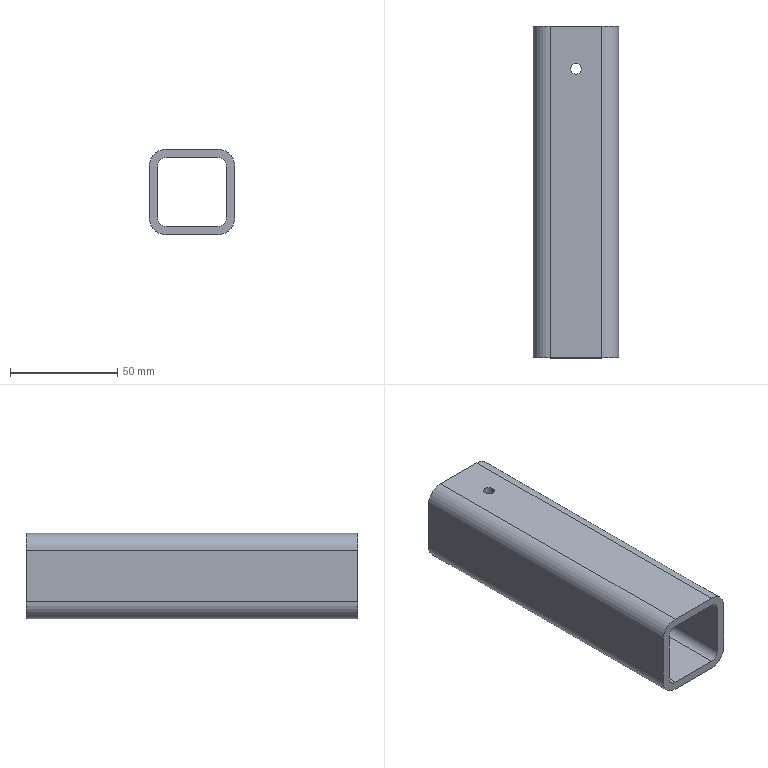Part | SolidWorks | features HoleWzd 1, WeldMemberFeat 1, WeldmentFeature 1 | 1 solid | 22 faces | box 40 x 155 x 40 mm | volume 82736 mm3 | cylinder 12 | plane 10 | commonest cylinder face diameters 5 x4 8 x4 16 x4
STEP:
#1=CARTESIAN_POINT('',(2.5,135.,16.));
#2=VERTEX_POINT('',#1);
#3=CARTESIAN_POINT('',(-2.5,135.,16.));
#4=VERTEX_POINT('',#3);
#5=CARTESIAN_POINT('',(0.,135.,16.));
#6=DIRECTION('',(0.,0.,-1.));
#7=DIRECTION('',(-1.,0.,0.));
#8=AXIS2_PLACEMENT_3D('',#5,#6,#7);
#9=CIRCLE('',#8,2.5);
#10=EDGE_CURVE('',#2,#4,#9,.T.);
#11=ORIENTED_EDGE('',*,*,#10,.T.);
#12=CARTESIAN_POINT('',(-2.5,135.,20.));
#13=VERTEX_POINT('',#12);
#14=CARTESIAN_POINT('',(-2.5,135.,20.));
#15=DIRECTION('',(0.,0.,1.));
#16=VECTOR('',#15,1000.);
#17=LINE('',#14,#16);
#18=EDGE_CURVE('',#4,#13,#17,.T.);
#19=ORIENTED_EDGE('',*,*,#18,.T.);
#20=CARTESIAN_POINT('',(2.5,135.,20.));
#21=VERTEX_POINT('',#20);
#22=CARTESIAN_POINT('',(0.,135.,20.));
#23=DIRECTION('',(0.,0.,1.));
#24=DIRECTION('',(1.,0.,0.));
#25=AXIS2_PLACEMENT_3D('',#22,#23,#24);
#26=CIRCLE('',#25,2.5);
#27=EDGE_CURVE('',#13,#21,#26,.T.);
#28=ORIENTED_EDGE('',*,*,#27,.T.);
#29=CARTESIAN_POINT('',(2.5,135.,20.));
#30=DIRECTION('',(0.,0.,1.));
#31=VECTOR('',#30,1000.);
#32=LINE('',#29,#31);
#33=EDGE_CURVE('',#2,#21,#32,.T.);
#34=ORIENTED_EDGE('',*,*,#33,.F.);
#35=EDGE_LOOP('',(#11,#19,#28,#34));
#36=FACE_OUTER_BOUND('',#35,.T.);
#37=CARTESIAN_POINT('',(0.,135.,20.));
#38=DIRECTION('',(0.,0.,1.));
#39=DIRECTION('',(1.,0.,0.));
#40=AXIS2_PLACEMENT_3D('',#37,#38,#39);
#41=CYLINDRICAL_SURFACE('',#40,2.5);
#42=ADVANCED_FACE('',(#36),#41,.F.);
#43=CARTESIAN_POINT('',(-2.5,135.,-20.));
#44=VERTEX_POINT('',#43);
#45=CARTESIAN_POINT('',(2.5,135.,-20.));
#46=VERTEX_POINT('',#45);
#47=CARTESIAN_POINT('',(0.,135.,-20.));
#48=DIRECTION('',(0.,0.,1.));
#49=DIRECTION('',(1.,0.,0.));
#50=AXIS2_PLACEMENT_3D('',#47,#48,#49);
#51=CIRCLE('',#50,2.5);
#52=EDGE_CURVE('',#44,#46,#51,.T.);
#53=ORIENTED_EDGE('',*,*,#52,.F.);
#54=CARTESIAN_POINT('',(-2.5,135.,-16.));
#55=VERTEX_POINT('',#54);
#56=CARTESIAN_POINT('',(-2.5,135.,20.));
#57=DIRECTION('',(0.,0.,1.));
#58=VECTOR('',#57,1000.);
#59=LINE('',#56,#58);
#60=EDGE_CURVE('',#44,#55,#59,.T.);
#61=ORIENTED_EDGE('',*,*,#60,.T.);
#62=CARTESIAN_POINT('',(2.5,135.,-16.));
#63=VERTEX_POINT('',#62);
#64=CARTESIAN_POINT('',(0.,135.,-16.));
#65=DIRECTION('',(0.,0.,1.));
#66=DIRECTION('',(1.,0.,0.));
#67=AXIS2_PLACEMENT_3D('',#64,#65,#66);
#68=CIRCLE('',#67,2.5);
#69=EDGE_CURVE('',#55,#63,#68,.T.);
#70=ORIENTED_EDGE('',*,*,#69,.T.);
#71=CARTESIAN_POINT('',(2.5,135.,20.));
#72=DIRECTION('',(0.,0.,1.));
#73=VECTOR('',#72,1000.);
#74=LINE('',#71,#73);
#75=EDGE_CURVE('',#46,#63,#74,.T.);
#76=ORIENTED_EDGE('',*,*,#75,.F.);
#77=EDGE_LOOP('',(#53,#61,#70,#76));
#78=FACE_OUTER_BOUND('',#77,.T.);
#79=CARTESIAN_POINT('',(0.,135.,20.));
#80=DIRECTION('',(0.,0.,1.));
#81=DIRECTION('',(1.,0.,0.));
#82=AXIS2_PLACEMENT_3D('',#79,#80,#81);
#83=CYLINDRICAL_SURFACE('',#82,2.5);
#84=ADVANCED_FACE('',(#78),#83,.F.);
#85=CARTESIAN_POINT('',(20.,155.,12.));
#86=VERTEX_POINT('',#85);
#87=CARTESIAN_POINT('',(12.,155.,20.));
#88=VERTEX_POINT('',#87);
#89=CARTESIAN_POINT('',(12.,155.,12.));
#90=DIRECTION('',(0.,-1.,0.));
#91=DIRECTION('',(1.,0.,0.));
#92=AXIS2_PLACEMENT_3D('',#89,#90,#91);
#93=CIRCLE('',#92,8.);
#94=EDGE_CURVE('',#86,#88,#93,.T.);
#95=ORIENTED_EDGE('',*,*,#94,.T.);
#96=CARTESIAN_POINT('',(12.,0.,20.));
#97=VERTEX_POINT('',#96);
#98=CARTESIAN_POINT('',(12.,0.,20.));
#99=DIRECTION('',(0.,1.,0.));
#100=VECTOR('',#99,1000.);
#101=LINE('',#98,#100);
#102=EDGE_CURVE('',#97,#88,#101,.T.);
#103=ORIENTED_EDGE('',*,*,#102,.F.);
#104=CARTESIAN_POINT('',(20.,0.,12.));
#105=VERTEX_POINT('',#104);
#106=CARTESIAN_POINT('',(12.,0.,12.));
#107=DIRECTION('',(0.,-1.,0.));
#108=DIRECTION('',(1.,0.,0.));
#109=AXIS2_PLACEMENT_3D('',#106,#107,#108);
#110=CIRCLE('',#109,8.);
#111=EDGE_CURVE('',#105,#97,#110,.T.);
#112=ORIENTED_EDGE('',*,*,#111,.F.);
#113=CARTESIAN_POINT('',(20.,0.,12.));
#114=DIRECTION('',(0.,1.,0.));
#115=VECTOR('',#114,1000.);
#116=LINE('',#113,#115);
#117=EDGE_CURVE('',#105,#86,#116,.T.);
#118=ORIENTED_EDGE('',*,*,#117,.T.);
#119=EDGE_LOOP('',(#95,#103,#112,#118));
#120=FACE_OUTER_BOUND('',#119,.T.);
#121=CARTESIAN_POINT('',(12.,0.,12.));
#122=DIRECTION('',(0.,1.,0.));
#123=DIRECTION('',(-1.,0.,0.));
#124=AXIS2_PLACEMENT_3D('',#121,#122,#123);
#125=CYLINDRICAL_SURFACE('',#124,8.);
#126=ADVANCED_FACE('',(#120),#125,.T.);
#127=CARTESIAN_POINT('',(0.,135.,20.));
#128=DIRECTION('',(0.,0.,1.));
#129=DIRECTION('',(1.,0.,0.));
#130=AXIS2_PLACEMENT_3D('',#127,#128,#129);
#131=CIRCLE('',#130,2.5);
#132=EDGE_CURVE('',#21,#13,#131,.T.);
#133=ORIENTED_EDGE('',*,*,#132,.F.);
#134=ORIENTED_EDGE('',*,*,#27,.F.);
#135=EDGE_LOOP('',(#133,#134));
#136=FACE_BOUND('',#135,.T.);
#137=CARTESIAN_POINT('',(-12.,155.,20.));
#138=VERTEX_POINT('',#137);
#139=CARTESIAN_POINT('',(12.,155.,20.));
#140=DIRECTION('',(-1.,0.,0.));
#141=VECTOR('',#140,1000.);
#142=LINE('',#139,#141);
#143=EDGE_CURVE('',#88,#138,#142,.T.);
#144=ORIENTED_EDGE('',*,*,#143,.T.);
#145=CARTESIAN_POINT('',(-12.,0.,20.));
#146=VERTEX_POINT('',#145);
#147=CARTESIAN_POINT('',(-12.,0.,20.));
#148=DIRECTION('',(0.,1.,0.));
#149=VECTOR('',#148,1000.);
#150=LINE('',#147,#149);
#151=EDGE_CURVE('',#146,#138,#150,.T.);
#152=ORIENTED_EDGE('',*,*,#151,.F.);
#153=CARTESIAN_POINT('',(12.,0.,20.));
#154=DIRECTION('',(-1.,0.,0.));
#155=VECTOR('',#154,1000.);
#156=LINE('',#153,#155);
#157=EDGE_CURVE('',#97,#146,#156,.T.);
#158=ORIENTED_EDGE('',*,*,#157,.F.);
#159=ORIENTED_EDGE('',*,*,#102,.T.);
#160=EDGE_LOOP('',(#144,#152,#158,#159));
#161=FACE_OUTER_BOUND('',#160,.T.);
#162=CARTESIAN_POINT('',(12.,0.,20.));
#163=DIRECTION('',(0.,0.,-1.));
#164=DIRECTION('',(-1.,0.,0.));
#165=AXIS2_PLACEMENT_3D('',#162,#163,#164);
#166=PLANE('',#165);
#167=ADVANCED_FACE('',(#136,#161),#166,.F.);
#168=CARTESIAN_POINT('',(-20.,155.,12.));
#169=VERTEX_POINT('',#168);
#170=CARTESIAN_POINT('',(-12.,155.,12.));
#171=DIRECTION('',(0.,-1.,0.));
#172=DIRECTION('',(1.,0.,0.));
#173=AXIS2_PLACEMENT_3D('',#170,#171,#172);
#174=CIRCLE('',#173,8.);
#175=EDGE_CURVE('',#138,#169,#174,.T.);
#176=ORIENTED_EDGE('',*,*,#175,.T.);
#177=CARTESIAN_POINT('',(-20.,0.,12.));
#178=VERTEX_POINT('',#177);
#179=CARTESIAN_POINT('',(-20.,0.,12.));
#180=DIRECTION('',(0.,1.,0.));
#181=VECTOR('',#180,1000.);
#182=LINE('',#179,#181);
#183=EDGE_CURVE('',#178,#169,#182,.T.);
#184=ORIENTED_EDGE('',*,*,#183,.F.);
#185=CARTESIAN_POINT('',(-12.,0.,12.));
#186=DIRECTION('',(0.,-1.,0.));
#187=DIRECTION('',(1.,0.,0.));
#188=AXIS2_PLACEMENT_3D('',#185,#186,#187);
#189=CIRCLE('',#188,8.);
#190=EDGE_CURVE('',#146,#178,#189,.T.);
#191=ORIENTED_EDGE('',*,*,#190,.F.);
#192=ORIENTED_EDGE('',*,*,#151,.T.);
#193=EDGE_LOOP('',(#176,#184,#191,#192));
#194=FACE_OUTER_BOUND('',#193,.T.);
#195=CARTESIAN_POINT('',(-12.,0.,12.));
#196=DIRECTION('',(0.,1.,0.));
#197=DIRECTION('',(-1.,0.,0.));
#198=AXIS2_PLACEMENT_3D('',#195,#196,#197);
#199=CYLINDRICAL_SURFACE('',#198,8.);
#200=ADVANCED_FACE('',(#194),#199,.T.);
#201=CARTESIAN_POINT('',(-20.,155.,-12.));
#202=VERTEX_POINT('',#201);
#203=CARTESIAN_POINT('',(-20.,155.,-12.));
#204=DIRECTION('',(0.,0.,-1.));
#205=VECTOR('',#204,1000.);
#206=LINE('',#203,#205);
#207=EDGE_CURVE('',#169,#202,#206,.T.);
#208=ORIENTED_EDGE('',*,*,#207,.T.);
#209=CARTESIAN_POINT('',(-20.,0.,-12.));
#210=VERTEX_POINT('',#209);
#211=CARTESIAN_POINT('',(-20.,0.,-12.));
#212=DIRECTION('',(0.,1.,0.));
#213=VECTOR('',#212,1000.);
#214=LINE('',#211,#213);
#215=EDGE_CURVE('',#210,#202,#214,.T.);
#216=ORIENTED_EDGE('',*,*,#215,.F.);
#217=CARTESIAN_POINT('',(-20.,0.,-12.));
#218=DIRECTION('',(0.,0.,-1.));
#219=VECTOR('',#218,1000.);
#220=LINE('',#217,#219);
#221=EDGE_CURVE('',#178,#210,#220,.T.);
#222=ORIENTED_EDGE('',*,*,#221,.F.);
#223=ORIENTED_EDGE('',*,*,#183,.T.);
#224=EDGE_LOOP('',(#208,#216,#222,#223));
#225=FACE_OUTER_BOUND('',#224,.T.);
#226=CARTESIAN_POINT('',(-20.,0.,-12.));
#227=DIRECTION('',(1.,0.,0.));
#228=DIRECTION('',(0.,1.,0.));
#229=AXIS2_PLACEMENT_3D('',#226,#227,#228);
#230=PLANE('',#229);
#231=ADVANCED_FACE('',(#225),#230,.F.);
#232=CARTESIAN_POINT('',(-12.,155.,-20.));
#233=VERTEX_POINT('',#232);
#234=CARTESIAN_POINT('',(-12.,155.,-12.));
#235=DIRECTION('',(0.,-1.,0.));
#236=DIRECTION('',(1.,0.,0.));
#237=AXIS2_PLACEMENT_3D('',#234,#235,#236);
#238=CIRCLE('',#237,8.);
#239=EDGE_CURVE('',#202,#233,#238,.T.);
#240=ORIENTED_EDGE('',*,*,#239,.T.);
#241=CARTESIAN_POINT('',(-12.,0.,-20.));
#242=VERTEX_POINT('',#241);
#243=CARTESIAN_POINT('',(-12.,0.,-20.));
#244=DIRECTION('',(0.,1.,0.));
#245=VECTOR('',#244,1000.);
#246=LINE('',#243,#245);
#247=EDGE_CURVE('',#242,#233,#246,.T.);
#248=ORIENTED_EDGE('',*,*,#247,.F.);
#249=CARTESIAN_POINT('',(-12.,0.,-12.));
#250=DIRECTION('',(0.,-1.,0.));
#251=DIRECTION('',(1.,0.,0.));
#252=AXIS2_PLACEMENT_3D('',#249,#250,#251);
#253=CIRCLE('',#252,8.);
#254=EDGE_CURVE('',#210,#242,#253,.T.);
#255=ORIENTED_EDGE('',*,*,#254,.F.);
#256=ORIENTED_EDGE('',*,*,#215,.T.);
#257=EDGE_LOOP('',(#240,#248,#255,#256));
#258=FACE_OUTER_BOUND('',#257,.T.);
#259=CARTESIAN_POINT('',(-12.,0.,-12.));
#260=DIRECTION('',(0.,1.,0.));
#261=DIRECTION('',(-1.,0.,0.));
#262=AXIS2_PLACEMENT_3D('',#259,#260,#261);
#263=CYLINDRICAL_SURFACE('',#262,8.);
#264=ADVANCED_FACE('',(#258),#263,.T.);
#265=CARTESIAN_POINT('',(0.,135.,-20.));
#266=DIRECTION('',(0.,0.,1.));
#267=DIRECTION('',(1.,0.,0.));
#268=AXIS2_PLACEMENT_3D('',#265,#266,#267);
#269=CIRCLE('',#268,2.5);
#270=EDGE_CURVE('',#46,#44,#269,.T.);
#271=ORIENTED_EDGE('',*,*,#270,.T.);
#272=ORIENTED_EDGE('',*,*,#52,.T.);
#273=EDGE_LOOP('',(#271,#272));
#274=FACE_BOUND('',#273,.T.);
#275=CARTESIAN_POINT('',(12.,155.,-20.));
#276=VERTEX_POINT('',#275);
#277=CARTESIAN_POINT('',(-12.,155.,-20.));
#278=DIRECTION('',(1.,0.,0.));
#279=VECTOR('',#278,1000.);
#280=LINE('',#277,#279);
#281=EDGE_CURVE('',#233,#276,#280,.T.);
#282=ORIENTED_EDGE('',*,*,#281,.T.);
#283=CARTESIAN_POINT('',(12.,0.,-20.));
#284=VERTEX_POINT('',#283);
#285=CARTESIAN_POINT('',(12.,0.,-20.));
#286=DIRECTION('',(0.,1.,0.));
#287=VECTOR('',#286,1000.);
#288=LINE('',#285,#287);
#289=EDGE_CURVE('',#284,#276,#288,.T.);
#290=ORIENTED_EDGE('',*,*,#289,.F.);
#291=CARTESIAN_POINT('',(-12.,0.,-20.));
#292=DIRECTION('',(1.,0.,0.));
#293=VECTOR('',#292,1000.);
#294=LINE('',#291,#293);
#295=EDGE_CURVE('',#242,#284,#294,.T.);
#296=ORIENTED_EDGE('',*,*,#295,.F.);
#297=ORIENTED_EDGE('',*,*,#247,.T.);
#298=EDGE_LOOP('',(#282,#290,#296,#297));
#299=FACE_OUTER_BOUND('',#298,.T.);
#300=CARTESIAN_POINT('',(-12.,0.,-20.));
#301=DIRECTION('',(0.,0.,1.));
#302=DIRECTION('',(1.,0.,0.));
#303=AXIS2_PLACEMENT_3D('',#300,#301,#302);
#304=PLANE('',#303);
#305=ADVANCED_FACE('',(#274,#299),#304,.F.);
#306=CARTESIAN_POINT('',(20.,155.,-12.));
#307=VERTEX_POINT('',#306);
#308=CARTESIAN_POINT('',(12.,155.,-12.));
#309=DIRECTION('',(0.,-1.,0.));
#310=DIRECTION('',(1.,0.,0.));
#311=AXIS2_PLACEMENT_3D('',#308,#309,#310);
#312=CIRCLE('',#311,8.);
#313=EDGE_CURVE('',#276,#307,#312,.T.);
#314=ORIENTED_EDGE('',*,*,#313,.T.);
#315=CARTESIAN_POINT('',(20.,0.,-12.));
#316=VERTEX_POINT('',#315);
#317=CARTESIAN_POINT('',(20.,0.,-12.));
#318=DIRECTION('',(0.,1.,0.));
#319=VECTOR('',#318,1000.);
#320=LINE('',#317,#319);
#321=EDGE_CURVE('',#316,#307,#320,.T.);
#322=ORIENTED_EDGE('',*,*,#321,.F.);
#323=CARTESIAN_POINT('',(12.,0.,-12.));
#324=DIRECTION('',(0.,-1.,0.));
#325=DIRECTION('',(1.,0.,0.));
#326=AXIS2_PLACEMENT_3D('',#323,#324,#325);
#327=CIRCLE('',#326,8.);
#328=EDGE_CURVE('',#284,#316,#327,.T.);
#329=ORIENTED_EDGE('',*,*,#328,.F.);
#330=ORIENTED_EDGE('',*,*,#289,.T.);
#331=EDGE_LOOP('',(#314,#322,#329,#330));
#332=FACE_OUTER_BOUND('',#331,.T.);
#333=CARTESIAN_POINT('',(12.,0.,-12.));
#334=DIRECTION('',(0.,1.,0.));
#335=DIRECTION('',(-1.,0.,0.));
#336=AXIS2_PLACEMENT_3D('',#333,#334,#335);
#337=CYLINDRICAL_SURFACE('',#336,8.);
#338=ADVANCED_FACE('',(#332),#337,.T.);
#339=CARTESIAN_POINT('',(-12.,155.,16.));
#340=VERTEX_POINT('',#339);
#341=CARTESIAN_POINT('',(-16.,155.,12.));
#342=VERTEX_POINT('',#341);
#343=CARTESIAN_POINT('',(-12.,155.,12.));
#344=DIRECTION('',(0.,-1.,0.));
#345=DIRECTION('',(1.,0.,0.));
#346=AXIS2_PLACEMENT_3D('',#343,#344,#345);
#347=CIRCLE('',#346,4.);
#348=EDGE_CURVE('',#340,#342,#347,.T.);
#349=ORIENTED_EDGE('',*,*,#348,.F.);
#350=CARTESIAN_POINT('',(-12.,0.,16.));
#351=VERTEX_POINT('',#350);
#352=CARTESIAN_POINT('',(-12.,0.,16.));
#353=DIRECTION('',(0.,1.,0.));
#354=VECTOR('',#353,1000.);
#355=LINE('',#352,#354);
#356=EDGE_CURVE('',#351,#340,#355,.T.);
#357=ORIENTED_EDGE('',*,*,#356,.F.);
#358=CARTESIAN_POINT('',(-16.,0.,12.));
#359=VERTEX_POINT('',#358);
#360=CARTESIAN_POINT('',(-12.,0.,12.));
#361=DIRECTION('',(0.,-1.,0.));
#362=DIRECTION('',(1.,0.,0.));
#363=AXIS2_PLACEMENT_3D('',#360,#361,#362);
#364=CIRCLE('',#363,4.);
#365=EDGE_CURVE('',#351,#359,#364,.T.);
#366=ORIENTED_EDGE('',*,*,#365,.T.);
#367=CARTESIAN_POINT('',(-16.,0.,12.));
#368=DIRECTION('',(0.,1.,0.));
#369=VECTOR('',#368,1000.);
#370=LINE('',#367,#369);
#371=EDGE_CURVE('',#359,#342,#370,.T.);
#372=ORIENTED_EDGE('',*,*,#371,.T.);
#373=EDGE_LOOP('',(#349,#357,#366,#372));
#374=FACE_OUTER_BOUND('',#373,.T.);
#375=CARTESIAN_POINT('',(-12.,0.,12.));
#376=DIRECTION('',(0.,1.,0.));
#377=DIRECTION('',(-1.,0.,0.));
#378=AXIS2_PLACEMENT_3D('',#375,#376,#377);
#379=CYLINDRICAL_SURFACE('',#378,4.);
#380=ADVANCED_FACE('',(#374),#379,.F.);
#381=ORIENTED_EDGE('',*,*,#10,.F.);
#382=CARTESIAN_POINT('',(0.,135.,16.));
#383=DIRECTION('',(0.,0.,-1.));
#384=DIRECTION('',(-1.,0.,0.));
#385=AXIS2_PLACEMENT_3D('',#382,#383,#384);
#386=CIRCLE('',#385,2.5);
#387=EDGE_CURVE('',#4,#2,#386,.T.);
#388=ORIENTED_EDGE('',*,*,#387,.F.);
#389=EDGE_LOOP('',(#381,#388));
#390=FACE_BOUND('',#389,.T.);
#391=CARTESIAN_POINT('',(12.,155.,16.));
#392=VERTEX_POINT('',#391);
#393=CARTESIAN_POINT('',(12.,155.,16.));
#394=DIRECTION('',(-1.,0.,0.));
#395=VECTOR('',#394,1000.);
#396=LINE('',#393,#395);
#397=EDGE_CURVE('',#392,#340,#396,.T.);
#398=ORIENTED_EDGE('',*,*,#397,.F.);
#399=CARTESIAN_POINT('',(12.,0.,16.));
#400=VERTEX_POINT('',#399);
#401=CARTESIAN_POINT('',(12.,0.,16.));
#402=DIRECTION('',(0.,1.,0.));
#403=VECTOR('',#402,1000.);
#404=LINE('',#401,#403);
#405=EDGE_CURVE('',#400,#392,#404,.T.);
#406=ORIENTED_EDGE('',*,*,#405,.F.);
#407=CARTESIAN_POINT('',(12.,0.,16.));
#408=DIRECTION('',(-1.,0.,0.));
#409=VECTOR('',#408,1000.);
#410=LINE('',#407,#409);
#411=EDGE_CURVE('',#400,#351,#410,.T.);
#412=ORIENTED_EDGE('',*,*,#411,.T.);
#413=ORIENTED_EDGE('',*,*,#356,.T.);
#414=EDGE_LOOP('',(#398,#406,#412,#413));
#415=FACE_OUTER_BOUND('',#414,.T.);
#416=CARTESIAN_POINT('',(12.,0.,16.));
#417=DIRECTION('',(0.,0.,-1.));
#418=DIRECTION('',(-1.,0.,0.));
#419=AXIS2_PLACEMENT_3D('',#416,#417,#418);
#420=PLANE('',#419);
#421=ADVANCED_FACE('',(#390,#415),#420,.T.);
#422=CARTESIAN_POINT('',(16.,155.,12.));
#423=VERTEX_POINT('',#422);
#424=CARTESIAN_POINT('',(12.,155.,12.));
#425=DIRECTION('',(0.,-1.,0.));
#426=DIRECTION('',(1.,0.,0.));
#427=AXIS2_PLACEMENT_3D('',#424,#425,#426);
#428=CIRCLE('',#427,4.);
#429=EDGE_CURVE('',#423,#392,#428,.T.);
#430=ORIENTED_EDGE('',*,*,#429,.F.);
#431=CARTESIAN_POINT('',(16.,0.,12.));
#432=VERTEX_POINT('',#431);
#433=CARTESIAN_POINT('',(16.,0.,12.));
#434=DIRECTION('',(0.,1.,0.));
#435=VECTOR('',#434,1000.);
#436=LINE('',#433,#435);
#437=EDGE_CURVE('',#432,#423,#436,.T.);
#438=ORIENTED_EDGE('',*,*,#437,.F.);
#439=CARTESIAN_POINT('',(12.,0.,12.));
#440=DIRECTION('',(0.,-1.,0.));
#441=DIRECTION('',(1.,0.,0.));
#442=AXIS2_PLACEMENT_3D('',#439,#440,#441);
#443=CIRCLE('',#442,4.);
#444=EDGE_CURVE('',#432,#400,#443,.T.);
#445=ORIENTED_EDGE('',*,*,#444,.T.);
#446=ORIENTED_EDGE('',*,*,#405,.T.);
#447=EDGE_LOOP('',(#430,#438,#445,#446));
#448=FACE_OUTER_BOUND('',#447,.T.);
#449=CARTESIAN_POINT('',(12.,0.,12.));
#450=DIRECTION('',(0.,1.,0.));
#451=DIRECTION('',(-1.,0.,0.));
#452=AXIS2_PLACEMENT_3D('',#449,#450,#451);
#453=CYLINDRICAL_SURFACE('',#452,4.);
#454=ADVANCED_FACE('',(#448),#453,.F.);
#455=CARTESIAN_POINT('',(16.,155.,-12.));
#456=VERTEX_POINT('',#455);
#457=CARTESIAN_POINT('',(16.,155.,12.));
#458=DIRECTION('',(0.,0.,1.));
#459=VECTOR('',#458,1000.);
#460=LINE('',#457,#459);
#461=EDGE_CURVE('',#456,#423,#460,.T.);
#462=ORIENTED_EDGE('',*,*,#461,.F.);
#463=CARTESIAN_POINT('',(16.,0.,-12.));
#464=VERTEX_POINT('',#463);
#465=CARTESIAN_POINT('',(16.,0.,-12.));
#466=DIRECTION('',(0.,1.,0.));
#467=VECTOR('',#466,1000.);
#468=LINE('',#465,#467);
#469=EDGE_CURVE('',#464,#456,#468,.T.);
#470=ORIENTED_EDGE('',*,*,#469,.F.);
#471=CARTESIAN_POINT('',(16.,0.,12.));
#472=DIRECTION('',(0.,0.,1.));
#473=VECTOR('',#472,1000.);
#474=LINE('',#471,#473);
#475=EDGE_CURVE('',#464,#432,#474,.T.);
#476=ORIENTED_EDGE('',*,*,#475,.T.);
#477=ORIENTED_EDGE('',*,*,#437,.T.);
#478=EDGE_LOOP('',(#462,#470,#476,#477));
#479=FACE_OUTER_BOUND('',#478,.T.);
#480=CARTESIAN_POINT('',(16.,0.,12.));
#481=DIRECTION('',(-1.,0.,0.));
#482=DIRECTION('',(0.,-1.,0.));
#483=AXIS2_PLACEMENT_3D('',#480,#481,#482);
#484=PLANE('',#483);
#485=ADVANCED_FACE('',(#479),#484,.T.);
#486=CARTESIAN_POINT('',(12.,155.,-16.));
#487=VERTEX_POINT('',#486);
#488=CARTESIAN_POINT('',(12.,155.,-12.));
#489=DIRECTION('',(0.,-1.,0.));
#490=DIRECTION('',(1.,0.,0.));
#491=AXIS2_PLACEMENT_3D('',#488,#489,#490);
#492=CIRCLE('',#491,4.);
#493=EDGE_CURVE('',#487,#456,#492,.T.);
#494=ORIENTED_EDGE('',*,*,#493,.F.);
#495=CARTESIAN_POINT('',(12.,0.,-16.));
#496=VERTEX_POINT('',#495);
#497=CARTESIAN_POINT('',(12.,0.,-16.));
#498=DIRECTION('',(0.,1.,0.));
#499=VECTOR('',#498,1000.);
#500=LINE('',#497,#499);
#501=EDGE_CURVE('',#496,#487,#500,.T.);
#502=ORIENTED_EDGE('',*,*,#501,.F.);
#503=CARTESIAN_POINT('',(12.,0.,-12.));
#504=DIRECTION('',(0.,-1.,0.));
#505=DIRECTION('',(1.,0.,0.));
#506=AXIS2_PLACEMENT_3D('',#503,#504,#505);
#507=CIRCLE('',#506,4.);
#508=EDGE_CURVE('',#496,#464,#507,.T.);
#509=ORIENTED_EDGE('',*,*,#508,.T.);
#510=ORIENTED_EDGE('',*,*,#469,.T.);
#511=EDGE_LOOP('',(#494,#502,#509,#510));
#512=FACE_OUTER_BOUND('',#511,.T.);
#513=CARTESIAN_POINT('',(12.,0.,-12.));
#514=DIRECTION('',(0.,1.,0.));
#515=DIRECTION('',(-1.,0.,0.));
#516=AXIS2_PLACEMENT_3D('',#513,#514,#515);
#517=CYLINDRICAL_SURFACE('',#516,4.);
#518=ADVANCED_FACE('',(#512),#517,.F.);
#519=CARTESIAN_POINT('',(0.,135.,-16.));
#520=DIRECTION('',(0.,0.,1.));
#521=DIRECTION('',(1.,0.,0.));
#522=AXIS2_PLACEMENT_3D('',#519,#520,#521);
#523=CIRCLE('',#522,2.5);
#524=EDGE_CURVE('',#63,#55,#523,.T.);
#525=ORIENTED_EDGE('',*,*,#524,.F.);
#526=ORIENTED_EDGE('',*,*,#69,.F.);
#527=EDGE_LOOP('',(#525,#526));
#528=FACE_BOUND('',#527,.T.);
#529=CARTESIAN_POINT('',(-12.,155.,-16.));
#530=VERTEX_POINT('',#529);
#531=CARTESIAN_POINT('',(-12.,155.,-16.));
#532=DIRECTION('',(1.,0.,0.));
#533=VECTOR('',#532,1000.);
#534=LINE('',#531,#533);
#535=EDGE_CURVE('',#530,#487,#534,.T.);
#536=ORIENTED_EDGE('',*,*,#535,.F.);
#537=CARTESIAN_POINT('',(-12.,0.,-16.));
#538=VERTEX_POINT('',#537);
#539=CARTESIAN_POINT('',(-12.,0.,-16.));
#540=DIRECTION('',(0.,1.,0.));
#541=VECTOR('',#540,1000.);
#542=LINE('',#539,#541);
#543=EDGE_CURVE('',#538,#530,#542,.T.);
#544=ORIENTED_EDGE('',*,*,#543,.F.);
#545=CARTESIAN_POINT('',(-12.,0.,-16.));
#546=DIRECTION('',(1.,0.,0.));
#547=VECTOR('',#546,1000.);
#548=LINE('',#545,#547);
#549=EDGE_CURVE('',#538,#496,#548,.T.);
#550=ORIENTED_EDGE('',*,*,#549,.T.);
#551=ORIENTED_EDGE('',*,*,#501,.T.);
#552=EDGE_LOOP('',(#536,#544,#550,#551));
#553=FACE_OUTER_BOUND('',#552,.T.);
#554=CARTESIAN_POINT('',(-12.,0.,-16.));
#555=DIRECTION('',(0.,0.,1.));
#556=DIRECTION('',(1.,0.,0.));
#557=AXIS2_PLACEMENT_3D('',#554,#555,#556);
#558=PLANE('',#557);
#559=ADVANCED_FACE('',(#528,#553),#558,.T.);
#560=CARTESIAN_POINT('',(-16.,155.,-12.));
#561=VERTEX_POINT('',#560);
#562=CARTESIAN_POINT('',(-12.,155.,-12.));
#563=DIRECTION('',(0.,-1.,0.));
#564=DIRECTION('',(1.,0.,0.));
#565=AXIS2_PLACEMENT_3D('',#562,#563,#564);
#566=CIRCLE('',#565,4.);
#567=EDGE_CURVE('',#561,#530,#566,.T.);
#568=ORIENTED_EDGE('',*,*,#567,.F.);
#569=CARTESIAN_POINT('',(-16.,0.,-12.));
#570=VERTEX_POINT('',#569);
#571=CARTESIAN_POINT('',(-16.,0.,-12.));
#572=DIRECTION('',(0.,1.,0.));
#573=VECTOR('',#572,1000.);
#574=LINE('',#571,#573);
#575=EDGE_CURVE('',#570,#561,#574,.T.);
#576=ORIENTED_EDGE('',*,*,#575,.F.);
#577=CARTESIAN_POINT('',(-12.,0.,-12.));
#578=DIRECTION('',(0.,-1.,0.));
#579=DIRECTION('',(1.,0.,0.));
#580=AXIS2_PLACEMENT_3D('',#577,#578,#579);
#581=CIRCLE('',#580,4.);
#582=EDGE_CURVE('',#570,#538,#581,.T.);
#583=ORIENTED_EDGE('',*,*,#582,.T.);
#584=ORIENTED_EDGE('',*,*,#543,.T.);
#585=EDGE_LOOP('',(#568,#576,#583,#584));
#586=FACE_OUTER_BOUND('',#585,.T.);
#587=CARTESIAN_POINT('',(-12.,0.,-12.));
#588=DIRECTION('',(0.,1.,0.));
#589=DIRECTION('',(-1.,0.,0.));
#590=AXIS2_PLACEMENT_3D('',#587,#588,#589);
#591=CYLINDRICAL_SURFACE('',#590,4.);
#592=ADVANCED_FACE('',(#586),#591,.F.);
#593=CARTESIAN_POINT('',(-16.,155.,-12.));
#594=DIRECTION('',(0.,0.,-1.));
#595=VECTOR('',#594,1000.);
#596=LINE('',#593,#595);
#597=EDGE_CURVE('',#342,#561,#596,.T.);
#598=ORIENTED_EDGE('',*,*,#597,.F.);
#599=ORIENTED_EDGE('',*,*,#371,.F.);
#600=CARTESIAN_POINT('',(-16.,0.,-12.));
#601=DIRECTION('',(0.,0.,-1.));
#602=VECTOR('',#601,1000.);
#603=LINE('',#600,#602);
#604=EDGE_CURVE('',#359,#570,#603,.T.);
#605=ORIENTED_EDGE('',*,*,#604,.T.);
#606=ORIENTED_EDGE('',*,*,#575,.T.);
#607=EDGE_LOOP('',(#598,#599,#605,#606));
#608=FACE_OUTER_BOUND('',#607,.T.);
#609=CARTESIAN_POINT('',(-16.,0.,-12.));
#610=DIRECTION('',(1.,0.,0.));
#611=DIRECTION('',(0.,1.,0.));
#612=AXIS2_PLACEMENT_3D('',#609,#610,#611);
#613=PLANE('',#612);
#614=ADVANCED_FACE('',(#608),#613,.T.);
#615=CARTESIAN_POINT('',(20.,155.,12.));
#616=DIRECTION('',(0.,0.,1.));
#617=VECTOR('',#616,1000.);
#618=LINE('',#615,#617);
#619=EDGE_CURVE('',#307,#86,#618,.T.);
#620=ORIENTED_EDGE('',*,*,#619,.T.);
#621=ORIENTED_EDGE('',*,*,#117,.F.);
#622=CARTESIAN_POINT('',(20.,0.,12.));
#623=DIRECTION('',(0.,0.,1.));
#624=VECTOR('',#623,1000.);
#625=LINE('',#622,#624);
#626=EDGE_CURVE('',#316,#105,#625,.T.);
#627=ORIENTED_EDGE('',*,*,#626,.F.);
#628=ORIENTED_EDGE('',*,*,#321,.T.);
#629=EDGE_LOOP('',(#620,#621,#627,#628));
#630=FACE_OUTER_BOUND('',#629,.T.);
#631=CARTESIAN_POINT('',(20.,0.,12.));
#632=DIRECTION('',(-1.,0.,0.));
#633=DIRECTION('',(0.,-1.,0.));
#634=AXIS2_PLACEMENT_3D('',#631,#632,#633);
#635=PLANE('',#634);
#636=ADVANCED_FACE('',(#630),#635,.F.);
#637=ORIENTED_EDGE('',*,*,#365,.F.);
#638=ORIENTED_EDGE('',*,*,#411,.F.);
#639=ORIENTED_EDGE('',*,*,#444,.F.);
#640=ORIENTED_EDGE('',*,*,#475,.F.);
#641=ORIENTED_EDGE('',*,*,#508,.F.);
#642=ORIENTED_EDGE('',*,*,#549,.F.);
#643=ORIENTED_EDGE('',*,*,#582,.F.);
#644=ORIENTED_EDGE('',*,*,#604,.F.);
#645=EDGE_LOOP('',(#637,#638,#639,#640,#641,#642,#643,#644));
#646=FACE_BOUND('',#645,.T.);
#647=ORIENTED_EDGE('',*,*,#111,.T.);
#648=ORIENTED_EDGE('',*,*,#157,.T.);
#649=ORIENTED_EDGE('',*,*,#190,.T.);
#650=ORIENTED_EDGE('',*,*,#221,.T.);
#651=ORIENTED_EDGE('',*,*,#254,.T.);
#652=ORIENTED_EDGE('',*,*,#295,.T.);
#653=ORIENTED_EDGE('',*,*,#328,.T.);
#654=ORIENTED_EDGE('',*,*,#626,.T.);
#655=EDGE_LOOP('',(#647,#648,#649,#650,#651,#652,#653,#654));
#656=FACE_OUTER_BOUND('',#655,.T.);
#657=CARTESIAN_POINT('',(12.,0.,12.));
#658=DIRECTION('',(0.,-1.,0.));
#659=DIRECTION('',(1.,0.,0.));
#660=AXIS2_PLACEMENT_3D('',#657,#658,#659);
#661=PLANE('',#660);
#662=ADVANCED_FACE('',(#646,#656),#661,.T.);
#663=ORIENTED_EDGE('',*,*,#348,.T.);
#664=ORIENTED_EDGE('',*,*,#597,.T.);
#665=ORIENTED_EDGE('',*,*,#567,.T.);
#666=ORIENTED_EDGE('',*,*,#535,.T.);
#667=ORIENTED_EDGE('',*,*,#493,.T.);
#668=ORIENTED_EDGE('',*,*,#461,.T.);
#669=ORIENTED_EDGE('',*,*,#429,.T.);
#670=ORIENTED_EDGE('',*,*,#397,.T.);
#671=EDGE_LOOP('',(#663,#664,#665,#666,#667,#668,#669,#670));
#672=FACE_BOUND('',#671,.T.);
#673=ORIENTED_EDGE('',*,*,#94,.F.);
#674=ORIENTED_EDGE('',*,*,#619,.F.);
#675=ORIENTED_EDGE('',*,*,#313,.F.);
#676=ORIENTED_EDGE('',*,*,#281,.F.);
#677=ORIENTED_EDGE('',*,*,#239,.F.);
#678=ORIENTED_EDGE('',*,*,#207,.F.);
#679=ORIENTED_EDGE('',*,*,#175,.F.);
#680=ORIENTED_EDGE('',*,*,#143,.F.);
#681=EDGE_LOOP('',(#673,#674,#675,#676,#677,#678,#679,#680));
#682=FACE_OUTER_BOUND('',#681,.T.);
#683=CARTESIAN_POINT('',(12.,155.,12.));
#684=DIRECTION('',(0.,-1.,0.));
#685=DIRECTION('',(1.,0.,0.));
#686=AXIS2_PLACEMENT_3D('',#683,#684,#685);
#687=PLANE('',#686);
#688=ADVANCED_FACE('',(#672,#682),#687,.F.);
#689=ORIENTED_EDGE('',*,*,#60,.F.);
#690=ORIENTED_EDGE('',*,*,#270,.F.);
#691=ORIENTED_EDGE('',*,*,#75,.T.);
#692=ORIENTED_EDGE('',*,*,#524,.T.);
#693=EDGE_LOOP('',(#689,#690,#691,#692));
#694=FACE_OUTER_BOUND('',#693,.T.);
#695=CARTESIAN_POINT('',(0.,135.,20.));
#696=DIRECTION('',(0.,0.,1.));
#697=DIRECTION('',(1.,0.,0.));
#698=AXIS2_PLACEMENT_3D('',#695,#696,#697);
#699=CYLINDRICAL_SURFACE('',#698,2.5);
#700=ADVANCED_FACE('',(#694),#699,.F.);
#701=ORIENTED_EDGE('',*,*,#18,.F.);
#702=ORIENTED_EDGE('',*,*,#387,.T.);
#703=ORIENTED_EDGE('',*,*,#33,.T.);
#704=ORIENTED_EDGE('',*,*,#132,.T.);
#705=EDGE_LOOP('',(#701,#702,#703,#704));
#706=FACE_OUTER_BOUND('',#705,.T.);
#707=CARTESIAN_POINT('',(0.,135.,20.));
#708=DIRECTION('',(0.,0.,1.));
#709=DIRECTION('',(1.,0.,0.));
#710=AXIS2_PLACEMENT_3D('',#707,#708,#709);
#711=CYLINDRICAL_SURFACE('',#710,2.5);
#712=ADVANCED_FACE('',(#706),#711,.F.);
#713=CLOSED_SHELL('',(#42,#84,#126,#167,#200,#231,#264,#305,#338,#380,#421,#454,#485,#518,#559,#592,#614,#636,#662,#688,#700,#712));
#714=MANIFOLD_SOLID_BREP('',#713);
#715=CARTESIAN_POINT('',(0.,0.,0.));
#716=DIRECTION('',(0.,0.,1.));
#717=DIRECTION('',(1.,0.,0.));
#718=AXIS2_PLACEMENT_3D('',#715,#716,#717);
#719=(LENGTH_UNIT()NAMED_UNIT(*)SI_UNIT(.MILLI.,.METRE.));
#720=UNCERTAINTY_MEASURE_WITH_UNIT(LENGTH_MEASURE(0.00001),#719,'','');
#721=(NAMED_UNIT(*)PLANE_ANGLE_UNIT()SI_UNIT($,.RADIAN.));
#722=(NAMED_UNIT(*)SI_UNIT($,.STERADIAN.)SOLID_ANGLE_UNIT());
#723=(GEOMETRIC_REPRESENTATION_CONTEXT(3)GLOBAL_UNCERTAINTY_ASSIGNED_CONTEXT((#720))GLOBAL_UNIT_ASSIGNED_CONTEXT((#719,#721,#722))REPRESENTATION_CONTEXT('',''));
#724=ADVANCED_BREP_SHAPE_REPRESENTATION('',(#714,#718),#723);